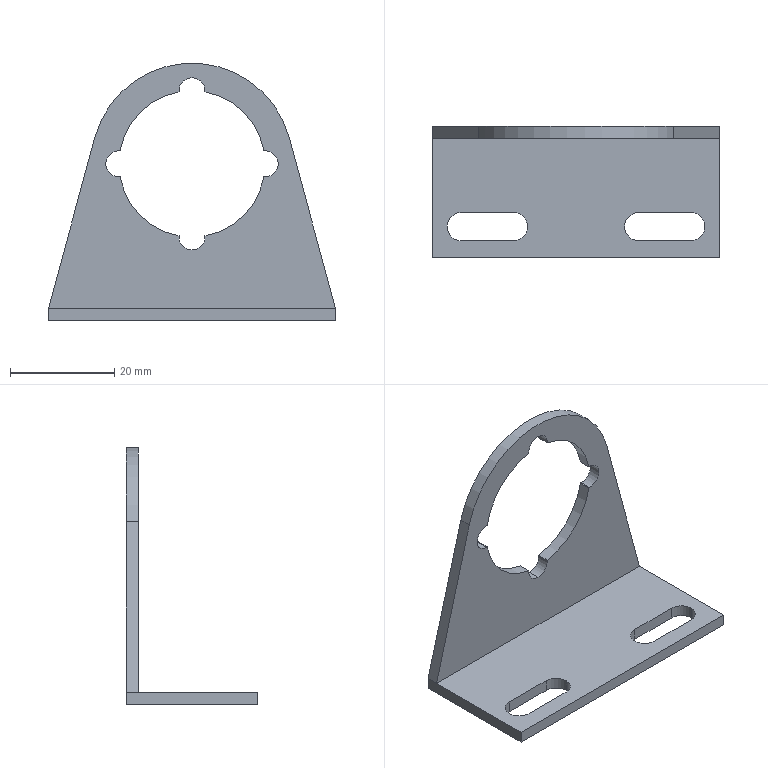Part | STEP file | 25A-AR20K-01B-D-Part-2 | 1 solid | 33 faces | box 55 x 25.2 x 49.3 mm | volume 5701 mm3 | cylinder 20 | plane 13 | commonest cylinder face diameters 5 x9 5.4 x6 28 x4 38.6 x1